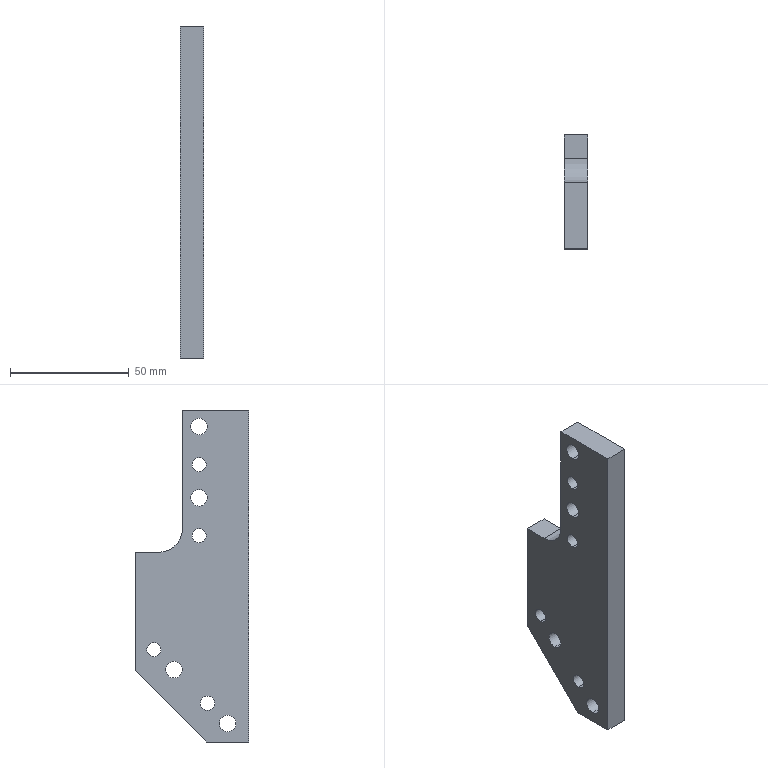Part | STEP file | OP10-156_side plate (F)-L | 1 solid | 26 faces | box 10 x 48 x 140 mm | volume 48244 mm3 | cylinder 17 | plane 9 | commonest cylinder face diameters 6 x8 7 x8 20 x1